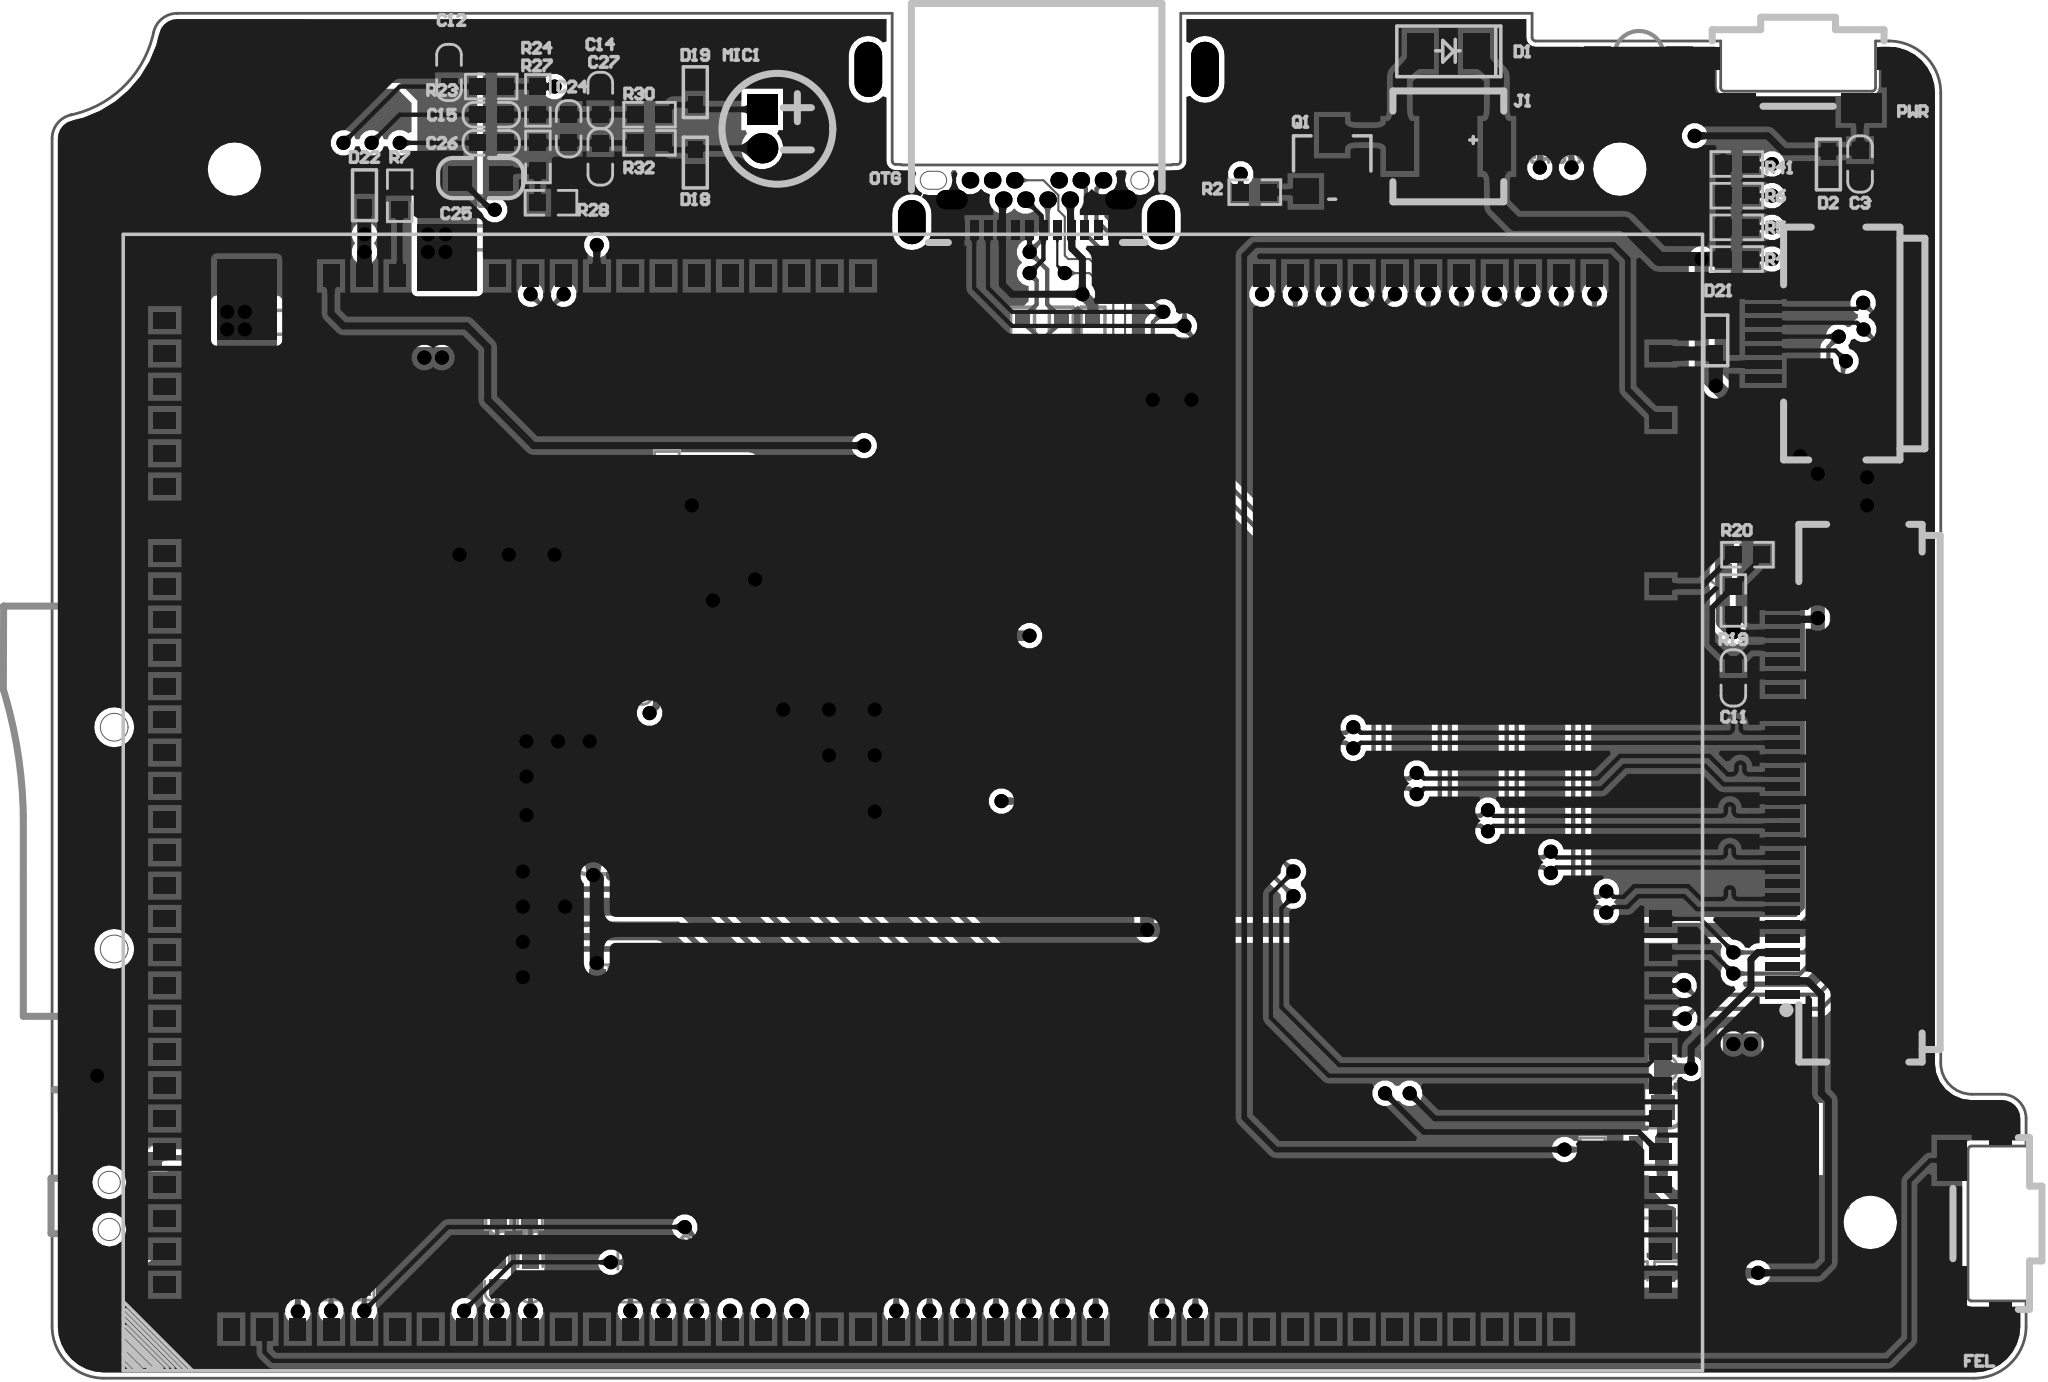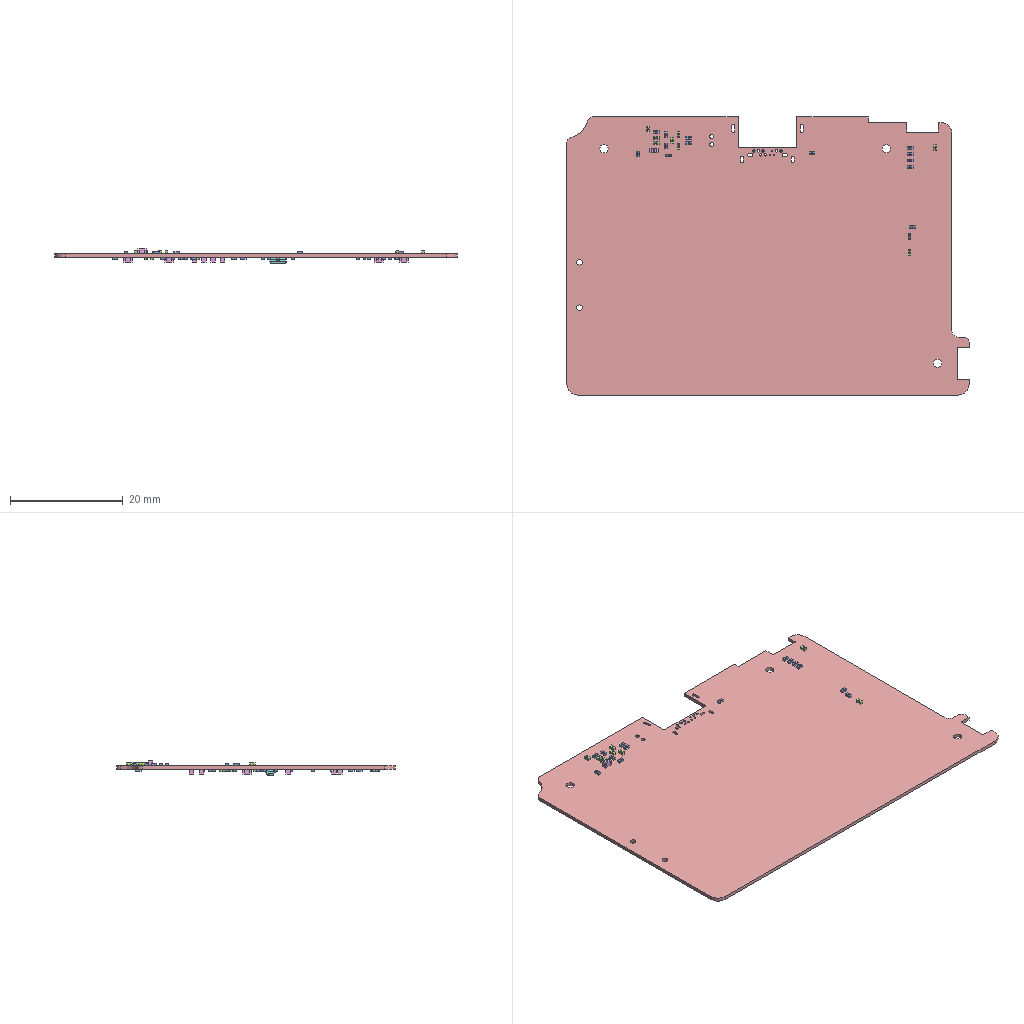Circuit board layout | Altium Designer | box 71.2 x 49.2 x 2.6 mm
Layer stack:
# Altium Designer layer stack of  (unit mm; dielectric type: 0 none, 1 core, 2 prepreg, 3 surface material)
index,name,kind,layer,copper_thickness_mm,dielectric_type,dielectric_thickness_mm,dielectric_material,dielectric_constant
0,Top Paste,other,,,,,,
1,Top Overlay,other,,,,,,
2,Top Solder,dielectric,,,3,0.0102,Solder Resist,3.5
3,Top Layer,copper,Top Layer,0.0356,,,,
4,Dielectric 2,dielectric,,,2,0.0711,PP-006,4.1
5,Layer 1,copper,Layer 1,0.035,,,,
6,Dielectric 1,dielectric,,,0,0.32,FR-4,4.8
7,Layer 2,copper,Layer 2,0.035,,,,
8,Dielectric 3,dielectric,,,2,0.0711,PP-006,4.1
9,Bottom Layer,copper,Bottom Layer,0.0356,,,,
10,Bottom Solder,dielectric,,,3,0.0102,Solder Resist,3.5
11,Bottom Overlay,other,,,,,,
12,Bottom Paste,other,,,,,,
# drill layer pairs: low layer,high layer
drill_pair,Top Layer,Bottom Layer
Part placement:
Designator,Comment,Layer,Footprint,Center-X(mm),Center-Y(mm),Rotation
RST,LXTD-0204-034,BottomLayer,SW-SMD_LXTD-0204-034,10.541,6.35,90
R41,R-472J,TopLayer,R0402,68.961,43.942,180
D19,AU0511P1,TopLayer,ESD0402A,31.369,46.533,270
D18,AU0511P1,TopLayer,ESD0402A,31.369,43.993,90
MIC1,GMI4015P-2C-64db,TopLayer,MIC-TH_BD4.0-P1.40-D0.4-L-FD,33.782,45.212,270
R40,R-103J,BottomLayer,R0402,32.766,24.003,0
R36,R-103J,BottomLayer,R0402,47.678,18.729,90
R32,R-304F,TopLayer,R0402,29.718,44.704,0
R30,R-104F,TopLayer,R0402,29.718,45.72,0
R29,R-103J,BottomLayer,R0402,39.878,23.749,0
R28,R-102,TopLayer,R0402,26.162,42.545,0
R27,R-152,TopLayer,R0402,25.689,44.2,90
R24,R-152,TopLayer,R0402,25.689,46.236,270
R23,R-102,TopLayer,R0402,24.003,46.736,180
D22,AU0511P1,TopLayer,ESD0402A,19.43,42.815,270
D21,AU0511P1,TopLayer,ESD0402A,68.2,37.576,90
D20,AU0511P1,BottomLayer,ESD0402A,23.606,41.276,0
C27,C-50-330,TopLayer,C0402,27.94,44.196,90
C26,C-50-104,TopLayer,C0402,24.003,44.704,0
C25,C-50-106,TopLayer,C0603,23.622,43.434,0
C24,C-50-101,TopLayer,C0402,26.797,45.212,90
C15,C-50-104,TopLayer,C0402,24.003,45.72,0
C14,C-50-330,TopLayer,C0402,27.94,46.236,270
C12,C-50-105,TopLayer,C0402,22.479,47.244,270
D17,AU0511P1,BottomLayer,ESD0402A,16.367,38.228,0
D16,SS34F_C18199199,BottomLayer,SMAF_L3.5-W2.6-LS4.7-RD-1,48.133,29.718,90
D15,SS34F_C18199199,BottomLayer,SMAF_L3.5-W2.6-LS4.7-RD-1,45.212,29.718,90
VIN-,Header 1,BottomLayer,HDR-LI-1P,15.24,31.369,90
VIN+,Header 1,BottomLayer,HDR-LI-1P,15.24,36.068,90
VBAT-,Header 1,BottomLayer,HDR-LI-1P,10.16,43.18,90
VBAT+,Header 1,BottomLayer,HDR-LI-1P,18.796,47.879,90
R39,R-5R0J,BottomLayer,R0402,50.292,23.368,90
R38,R-103J,BottomLayer,R0402,45.085,23.368,90
R37,R-103J,BottomLayer,R0402,46.228,25.019,180
Q3,8050-S,BottomLayer,SOT-23-3,47.691,22.168,270
U1,TPS61089RNRR,BottomLayer,VQFN-HR_L2.5-W2.0-P0.50-TL-EP,30.218,27.432,270
L2,FXL0518-2R2-M,BottomLayer,IND-SMD_L5.2-W5.4,24.638,29.845,270
U8,MT9700,BottomLayer,SOT-23-5_L3.0-W1.7-P0.95-LS2.8-BR,40.797,25.974,0
R35,R-622F,BottomLayer,R0402,32.377,30.353,90
R34,R-154J,BottomLayer,R0402,30.734,24.511,90
R33,R-332J,BottomLayer,R0402,41.529,28.448,0
R31,R-202J,BottomLayer,R0402,61.849,45.593,90
R26,R-202J,BottomLayer,R0402,62.992,45.593,90
R25,R-104F,BottomLayer,R0402,28.694,32.131,180
R3,R-304F,BottomLayer,R0402,30.345,32.639,90
R1,R-304J,BottomLayer,R0402,28.694,29.845,0
FEL,TSB017A3126A02,TopLayer,KEY-SMD_YTSB017A0312502B,77.597,5.715,90
LED1,XL-3210SURUGC,BottomLayer,LED-SMD_4P-L3.2-W1.5_HTG-3210SURUBGC,65.405,47.498,180
C23,C-16-106(±10%),BottomLayer,C0603,32.885,26.32,90
C22,C-16-106(±10%),BottomLayer,C0603,34.536,26.32,90
C21,C-16-106(±10%),BottomLayer,C0603,36.187,26.289,90
C20,C-50-220(±10%),BottomLayer,C0402,33.52,30.353,90
C19,C-16-106(±10%),BottomLayer,C0603,37.838,26.289,90
C18,C-50-472(±10%),BottomLayer,C0402,31.234,30.353,270
C17,C-16-106(±10%),BottomLayer,C0603,21.082,34.417,0
C16,C-16-106(±10%),BottomLayer,C0603,21.082,36.195,0
C2,C-50-104(±10%),BottomLayer,C0402,28.829,24.892,0
C1,C-16-225(±10%),BottomLayer,C0402,28.694,30.988,180
OTG,GT-USB-9009B,TopLayer,USB-C-SMD_GT-USB-9009B,43.688,44.45,180
PWR,TSB017A3126A02,TopLayer,KEY-SMD_YTSB017A0312502B,71.171,46.863,180
ESD18,AU0511P1,BottomLayer,ESD0402A,62.485,37.862,270
ESD17,AU0511P1,BottomLayer,ESD0402A,63.983,37.862,270
ESD16,AU0511P1,BottomLayer,ESD0402A,60.072,35.83,270
ESD15,AU0511P1,BottomLayer,ESD0402A,61.596,35.83,270
ESD14,AU0511P1,BottomLayer,ESD0402A,57.659,37.862,270
ESD13,AU0511P1,BottomLayer,ESD0402A,59.183,37.862,270
ESD12,AU0511P1,BottomLayer,ESD0402A,55.246,35.83,270
ESD11,AU0511P1,BottomLayer,ESD0402A,56.812,35.83,270
ESD10,AU0511P1,BottomLayer,ESD0402A,52.874,37.862,270
ESD9,AU0511P1,BottomLayer,ESD0402A,54.357,37.862,270
ESD8,AU0511P1,BottomLayer,ESD0402A,73.153,33.925,270
ESD7,AU0511P1,BottomLayer,ESD0402A,71.883,33.925,270
ESD6,AU0511P1,BottomLayer,ESD0402A,74.169,33.925,270
ESD5,AU0511P1,BottomLayer,ESD0402A,75.566,33.925,270
U2,HelperA133Core,TopLayer,A133_-_duplicate,39.221,20.905,90
FPC1,AFC01-S08FCA-00,TopLayer,FPC-SMD_P0.50-8P_FGS-XJ-H2.0,71.247,37.465,270
U4,xc6206p182mr,BottomLayer,SOT23,69.342,31.648,180
U3,HM5663,BottomLayer,SOT23-6,66.267,6.858,270
L1,10uH,BottomLayer,IND-SMD_L2.5-W2.0,70.231,8.763,180
J2,TF-115-BCP9,BottomLayer,TF-SMD_TF-115-BCP9,16.095,20.571,90
J1,FUET-4020,TopLayer,BUZ-SMD_L4.0-W4.0-P3.50-L,58.547,44.577,180
R22,R-103J,BottomLayer,R0402,27.321,14.604,180
R21,R-103J,BottomLayer,R0402,27.305,21.209,180
R20,R-0J,TopLayer,R0402,69.342,29.845,0
R19,R-103J,TopLayer,R0402,68.834,28.194,90
R18,8R2,BottomLayer,R0402,65.288,3.408,270
R17,8R2,BottomLayer,R0402,66.431,3.408,270
R16,8R2,BottomLayer,R0402,67.574,3.408,270
R15,1M,BottomLayer,R0402,63.754,7.874,270
R14,NC,BottomLayer,R0402,68.707,3.429,270
R6,R-472J,TopLayer,R0402,68.961,42.799,180
R5,R-472J,TopLayer,R0402,68.961,41.656,180
R4,R-472J,TopLayer,R0402,68.961,40.513,180
Q1,S9013,TopLayer,SOT23,54.356,43.967,0
FPC2,FPC-05F-30PH20,TopLayer,FPC-SMD_30P-P0.50_XUNPU_FPC-05F-30PH20,72.147,21.241,90
ESD2,AU0511P1,BottomLayer,ESD0402A,49.277,36.719,270
ESD1,AU0511P1,BottomLayer,ESD0402A,47.88,36.719,270
D14,AU0511P1,BottomLayer,ESD0402A,45.721,37.862,270
D13,AU0511P1,BottomLayer,ESD0402A,44.578,37.862,270
D12,AU0511P1,BottomLayer,ESD0402A,23.987,21.845,0
D11,AU0511P1,BottomLayer,ESD0402A,23.987,20.575,0
D10,AU0511P1,BottomLayer,ESD0402A,24.003,18.415,0
D9,AU0511P1,BottomLayer,ESD0402A,24.003,17.145,0
D8,AU0511P1,BottomLayer,ESD0402A,24.003,15.875,0
D7,AU0511P1,BottomLayer,ESD0402A,23.987,23.115,0
D6,AU0511P1,BottomLayer,ESD0402A,26.304,19.541,90
D5,AU0511P1,BottomLayer,ESD0402A,24.003,14.605,0
D4,1N5819,BottomLayer,SOD323,70.231,6.477,180
D3,AU0511P1,BottomLayer,ESD0402A,43.181,37.862,270
D2,AU0511P1,TopLayer,ESD0402A,72.264,43.926,90
D1,1N5819,TopLayer,SOD323,58.547,48.006,0
C13,C-25-106,BottomLayer,C0603,28.448,19.05,180
C11,C-25-104,TopLayer,C0402,68.834,25.4,270
C10,C-25-104,BottomLayer,C0402,68.961,29.21,0
C9,C-25-104,BottomLayer,C0402,68.834,34.163,180
C8,C-25-106,BottomLayer,C0603,69.977,10.922,0
C7,C-25-104,BottomLayer,C0402,65.786,11.303,0
C6,C-25-106,BottomLayer,C0603,65.532,9.906,180
R12,R-105J,BottomLayer,R0402,31.414,3.81,270
R13,R-104J,BottomLayer,R0402,18.84,3.397,180
R9,R-202J,BottomLayer,R0402,29.019,3.81,90
R8,R-0J,BottomLayer,R0402,30.226,3.81,270
R2,R-152J,TopLayer,R0402,51.562,42.926,0
R7,R-103J,TopLayer,R0402,20.701,42.799,270
R11,R-220J,BottomLayer,R0402,25.4,6.477,270
R10,R-220J,BottomLayer,R0402,24.257,6.469,90
C3,C-25-104,TopLayer,C0402,73.406,43.942,90
C5,C-25-104,BottomLayer,C0402,25.418,3.896,270
C4,C-25-104,BottomLayer,C0402,24.212,3.896,270
Pad and via stacks:
# Altium Designer via and pad stacks of  (unit mm). Each distinct definition once, with the count of objects using it.
# via: kind,start_layer,end_layer,hole_mm,diameter_mm,mode(0 simple;1 top-mid-bottom;2 full stack),diameter_per_layer,count,example_net
# pad: kind,layer,hole_mm,hole_type(0 round;1 square;2 slot),plating,top_size,top_shape(1 round;2 rect;3 octagon;9 rounded rect),mid_size,bottom_size,mode,footprint,size_per_layer,count,example
pad,Top Layer,0,0,plated,0.3x0.7,2,0.3x0.7,0.3x0.7,0,USB-C-SMD_GT-USB-9009B,,12,OTG.A12
pad,Top Layer,0,0,plated,1.27x0.9398,2,1.27x0.9398,1.27x0.9398,0,SOD323,,2,D1.2
pad,Top Layer,0,0,plated,0.6x0.6,2,0.6x0.6,0.6x0.6,0,R0402,,28,R41.2
pad,Top Layer,0,0,plated,0.6x0.6,2,0.6x0.6,0.6x0.6,0,C0402,,16,C12.1
pad,Top Layer,0,0,plated,0.6096x0.508,2,0.6096x0.508,0.6096x0.508,0,ESD0402A,,10,D19.1
pad,Top Layer,0,0,plated,0.9x0.85,2,0.9x0.85,0.9x0.85,0,C0603,,2,C25.1
pad,Top Layer,0,0,plated,0.8x0.6096,2,0.8x0.6096,0.8x0.6096,0,A133 - duplicate,,121,U2.31
pad,Top Layer,0,0,plated,0.65x0.8,2,0.65x0.8,0.65x0.8,0,KEY-SMD_YTSB017A0312502B,,4,FEL.4
pad,Top Layer,0,0,plated,1.45x1.05,2,1.45x1.05,1.45x1.05,0,KEY-SMD_YTSB017A0312502B,,4,FEL.2
pad,Top Layer,0,0,plated,1x1.8,2,1x1.8,1x1.8,0,BUZ-SMD_L4.0-W4.0-P3.50-L,,2,J1.2
pad,Top Layer,0,0,plated,0.9144x0.9144,2,0.9144x0.9144,0.9144x0.9144,0,SOT23,,2,Q1.1
pad,Top Layer,0,0,plated,1.27x0.9144,2,1.27x0.9144,1.27x0.9144,0,SOT23,,1,Q1.3
pad,Top Layer,0,0,plated,1.6x2,2,1.6x2,1.6x2,0,FPC-SMD_P0.50-8P_FGS-XJ-H2.0,,2,FPC1.10
pad,Top Layer,0,0,plated,0.3x1.3,2,0.3x1.3,0.3x1.3,0,FPC-SMD_P0.50-8P_FGS-XJ-H2.0,,8,FPC1.1
pad,Top Layer,0,0,plated,2x2.5,2,2x2.5,2x2.5,0,FPC-SMD_30P-P0.50_XUNPU_FPC-05F-30PH20,,2,FPC2.31
pad,Top Layer,0,0,plated,0.3x1.25,2,0.3x1.25,0.3x1.25,0,FPC-SMD_30P-P0.50_XUNPU_FPC-05F-30PH20,,30,FPC2.30
pad,Bottom Layer,0,0,plated,0.21x0.21,1,0.21x0.21,0.21x0.21,0,SW-SMD_LXTD-0204-034,,2,RST.3
pad,Bottom Layer,0,0,plated,0.5x1.2,2,0.5x1.2,0.5x1.2,0,SW-SMD_LXTD-0204-034,,2,RST.1
pad,Bottom Layer,0,0,plated,0.6096x0.508,2,0.6096x0.508,0.6096x0.508,0,ESD0402A,,58,ESD7.1
pad,Bottom Layer,0,0,plated,0.6x0.6,2,0.6x0.6,0.6x0.6,0,R0402,,54,R40.2
pad,Bottom Layer,0,0,plated,1.524x1.524,9,1.524x1.524,1.524x1.524,0,HDR-LI-1P,,4,VBAT+.1
pad,Bottom Layer,0,0,plated,1.9x2.5,2,1.9x2.5,1.9x2.5,0,IND-SMD_L5.2-W5.4,,2,L2.2
pad,Bottom Layer,0,0,plated,1.1x1.1,2,1.1x1.1,1.1x1.1,0,VQFN-HR_L2.5-W2.0-P0.50-TL-EP,,1,U1.11
pad,Bottom Layer,0,0,plated,0.9x0.85,2,0.9x0.85,0.9x0.85,0,C0603,,18,C8.1
pad,Bottom Layer,0,0,plated,1.2x2.2,2,1.2x2.2,1.2x2.2,0,IND-SMD_L2.5-W2.0,,2,L1.1
pad,Bottom Layer,0,0,plated,0.3x0.6,2,0.3x0.6,0.3x0.6,0,VQFN-HR_L2.5-W2.0-P0.50-TL-EP,,8,U1.9
pad,Bottom Layer,0,0,unplated,1.2x0.5,2,1.2x0.5,1.2x0.5,0,SOT23-6,,6,U3.6
pad,Bottom Layer,0,0,plated,0.8x1.6,2,0.8x1.6,0.8x1.6,0,SOT-23-3,,3,Q3.3
pad,Bottom Layer,0,0,plated,0.6x0.6,2,0.6x0.6,0.6x0.6,0,C0402,,18,C20.2
pad,Bottom Layer,0,0,plated,0.45x1.2,2,0.45x1.2,0.45x1.2,0,VQFN-HR_L2.5-W2.0-P0.50-TL-EP,,2,U1.5
pad,Bottom Layer,0,0,plated,1.1x0.6,2,1.1x0.6,1.1x0.6,0,SOT-23-5_L3.0-W1.7-P0.95-LS2.8-BR,,5,U8.5
pad,Bottom Layer,0,0,plated,0.95x1.1,2,0.95x1.1,0.95x1.1,0,LED-SMD_4P-L3.2-W1.5_HTG-3210SURUBGC,,2,LED1.3
pad,Bottom Layer,0,0,plated,0.5001x0.6,2,0.5001x0.6,0.5001x0.6,0,LED-SMD_4P-L3.2-W1.5_HTG-3210SURUBGC,,2,LED1.1
pad,Bottom Layer,0,0,plated,1.6x1.7,2,1.6x1.7,1.6x1.7,0,SMAF_L3.5-W2.6-LS4.7-RD-1,,4,D16.1
pad,Bottom Layer,0,0,plated,0.7x1.6,2,0.7x1.6,0.7x1.6,0,TF-SMD_TF-115-BCP9,,9,J2.1
pad,Bottom Layer,0,0,plated,1.2x1.5,2,1.2x1.5,1.2x1.5,0,TF-SMD_TF-115-BCP9,,1,J2.10
pad,Bottom Layer,0,0,plated,1.2x2.2,2,1.2x2.2,1.2x2.2,0,TF-SMD_TF-115-BCP9,,2,J2.11
pad,Bottom Layer,0,0,plated,1.6x1.5,2,1.6x1.5,1.6x1.5,0,TF-SMD_TF-115-BCP9,,1,J2.12
pad,Bottom Layer,0,0,plated,1.27x0.9398,2,1.27x0.9398,1.27x0.9398,0,SOD323,,2,D4.1
pad,Bottom Layer,0,0,plated,1.27x0.9144,2,1.27x0.9144,1.27x0.9144,0,SOT23,,1,U4.3
pad,Bottom Layer,0,0,plated,0.9144x0.9144,2,0.9144x0.9144,0.9144x0.9144,0,SOT23,,2,U4.2
pad,Multi-Layer,0.5,2,plated,0.7x1.15,1,0.7x1.15,0.7x1.15,0,USB-C-SMD_GT-USB-9009B,,2,OTG.B12
pad,Multi-Layer,0.4,0,plated,0.6x0.6,1,0.6x0.6,0.6x0.6,0,USB-C-SMD_GT-USB-9009B,,7,OTG.B2
pad,Multi-Layer,0.25,0,plated,0.6x0.6,1,0.6x0.6,0.6x0.6,0,USB-C-SMD_GT-USB-9009B,,3,OTG.B8
pad,Multi-Layer,0.5,2,plated,1x1.6,1,1x1.6,1x1.6,0,USB-C-SMD_GT-USB-9009B,,2,OTG.5
pad,Multi-Layer,0.5,2,plated,1x2,1,1x2,1x2,0,USB-C-SMD_GT-USB-9009B,,2,OTG.4
pad,Multi-Layer,0.7,0,plated,1.1x1.1,2,1.1x1.1,1.1x1.1,0,MIC-TH_BD4.0-P1.40-D0.4-L-FD,,1,MIC1.1
pad,Multi-Layer,0.7,0,plated,1.1x1.1,1,1.1x1.1,1.1x1.1,0,MIC-TH_BD4.0-P1.40-D0.4-L-FD,,1,MIC1.2
via,Top Layer,Bottom Layer,0.254,0.508,0,,140,GND
Copper pours:
name,layer,net,type(0 solid;1 hatched;2 none)
GND_L01_P001,Top Layer,GND,0
GND_L02_P002,Layer 1,GND,0
GND_L04_P003,Bottom Layer,GND,0
VCC_PS_L03_P004,Layer 2,VCC_PS,0
Design rules, without the lines most boards share:
# Altium Designer design rules of  (exported by Altium Designer, unit mm)
# columns: name | kind | enabled | priority | scope1 | scope2 | descriptor | typed fields (field=value)
DiffPairsRouting | 51 | enabled | 1 | InDifferentialPairClass('D_90om') | All | Differential Pairs Uncoupled Length using the Gap Constraints (Min=0.203mm) (Max=0.254mm) (Prefered=0.203mm)  and Width Constraints (Min=0.158mm) (Max=0.158mm) (Prefered=0.158mm) (InDifferentialPairClass('D_90om')) |
NetAntennae | 56 | enabled | 1 | All | All | Net Antennae (Tolerance=0mm) (All) |
SilkToSilkClearance | 55 | enabled | 1 | All | All | Silk to Silk (Clearance=0mm) (All),(All) |
SilkToSolderMaskClearance | 54 | enabled | 1 | IsPad | All | Silk To Solder Mask (Clearance=0mm) (IsPad),(All) |
MinimumSolderMaskSliver | 53 | enabled | 1 | All | All | Minimum Solder Mask Sliver (Gap=0mm) (All),(All) |
HoleToHoleClearance | 52 | enabled | 1 | All | All | Hole To Hole Clearance (Gap=0.254mm) (All),(All) | gap=0.254
HoleSize | 42 | enabled | 1 | All | All | Hole Size Constraint (Min=0.025mm) (Max=2.54mm) (All) |
Height | 50 | enabled | 1 | All | All | Height Constraint (Min=0mm) (Max=25.4mm) (Prefered=12.7mm) (All) | min_height=0 max_height=25.4
ComponentClearance | 24 | enabled | 1 | All | All | Component Clearance Constraint ( Horizontal Gap = 0mm, Vertical Gap = 0mm ) (All),(All)  | gap=0
SolderMaskExpansion | 13 | enabled | 1 | All | All | Solder Mask Expansion (Expansion =0.102mm) (All) | expansion=0.1016
PasteMaskExpansion | 14 | enabled | 1 | All | All | Paste Mask Expansion (Expansion =0mm) (All) | expansion=0
RoutingVias | 11 | enabled | 1 | All | All | Routing Via (MinHoleWidth=0.254mm) (MaxHoleWidth=0.254mm) (PreferredHoleWidth=0.254mm) (MinWidth=0.508mm) (MaxWidth=0.508mm) (PreferedWidth=0.508mm) (All) | via_min_hole=0.254 via_max_hole=0.254 via_preferred_diameter=0.508 via_preferred_hole=0.254
RoutingCorners | 10 | enabled | 1 | All | All | Routing Corners (Style=45-Degree) (Min Setback=2.54mm) (Max Setback=2.54mm) (All) |
Width | 2 | enabled | 1 | All | All | Width Constraint (Min=0.025mm) (Max=1.27mm) (Preferred=0.254mm) (All) |
PolygonConnect | 20 | enabled | 1 | All | All | Polygon Connect Rule(Direct Connect )(Conductor Width=0.254mm) (Relief Angle=90 Angle) (Entries=4) (Air Gap Width=0.254mm) (All),(All) | connect_style(0=relief,1=direct,2=none)=1 relief_conductor_width=0.254 relief_entries=4
PlaneClearance | 12 | enabled | 1 | All | All | Power Plane Clearance (Clearance =0.508mm) (All) | clearance=0.508
PlaneConnect | 6 | enabled | 1 | All | All | Power Plane Connect Rule(Relief Connect )(Expansion=0.508mm) (Conductor Width=0.254mm) (Air Gap=0.254mm) (Entries=4) (All) | relief_conductor_width=0.254 relief_entries=4 relief_expansion=0.508
Clearance | 0 | enabled | 1 | All | All | Clearance Constraint (Gap=0.051mm) (All),(All) | gap=0.0508
Classes set for this board:
# Altium Designer classes of  (member kind: 0 net, 1 component, 2 from-to, 3 pad, 4 layer, 5 differential pair, 6 design channel, 7 polygon, 8 structure, 9 xSignal)
# columns: class name | member kind | superclass | members
D_90om | 6 | no | MIPI_CL; MIPI_D0; MIPI_D1; MIPI_D2; MIPI_D3; USB0; MICIN1;